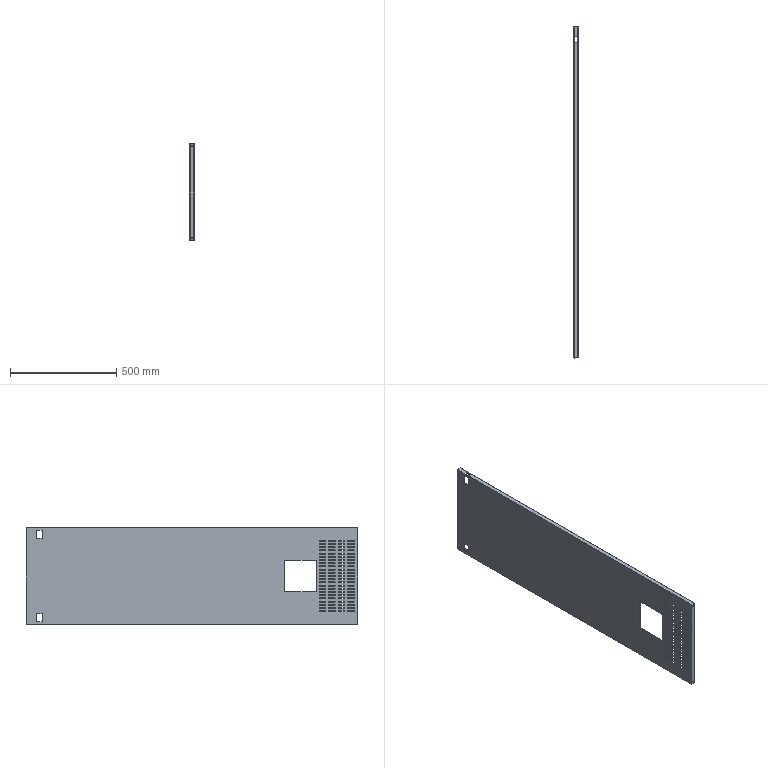Part | SolidWorks | features SplitBody 1 | 1 solid | 462 faces | box 20 x 1560 x 458 mm | volume 785912 mm3 | plane 240 | cylinder 206 | spline 16 | commonest cylinder face diameters 5 x184 0.2 x10 2.2 x8 4.5 x4